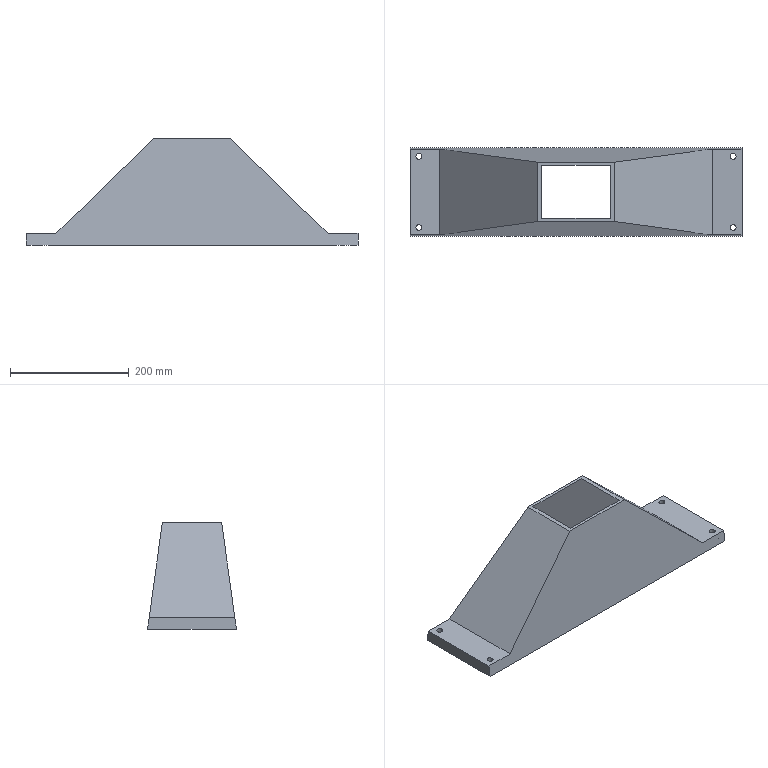Part | SolidWorks | features BaseBody 1 | 1 solid | 34 faces | box 560 x 150 x 180 mm | volume 1083065 mm3 | plane 18 | cylinder 16 | commonest cylinder face diameters 10 x8 25 x8
STEP:
#1=CARTESIAN_POINT('',(260.,-60.,20.));
#2=VERTEX_POINT('',#1);
#3=CARTESIAN_POINT('',(270.,-60.,20.));
#4=VERTEX_POINT('',#3);
#5=CARTESIAN_POINT('',(265.,-60.,20.));
#6=DIRECTION('',(0.,0.,-1.));
#7=DIRECTION('',(1.,0.,0.));
#8=AXIS2_PLACEMENT_3D('',#5,#6,#7);
#9=CIRCLE('',#8,5.);
#10=EDGE_CURVE('',#2,#4,#9,.T.);
#11=ORIENTED_EDGE('',*,*,#10,.F.);
#12=CARTESIAN_POINT('',(260.,-60.,10.));
#13=VERTEX_POINT('',#12);
#14=CARTESIAN_POINT('',(260.,-60.,10.));
#15=DIRECTION('',(0.,0.,-1.));
#16=VECTOR('',#15,1000.);
#17=LINE('',#14,#16);
#18=EDGE_CURVE('',#2,#13,#17,.T.);
#19=ORIENTED_EDGE('',*,*,#18,.T.);
#20=CARTESIAN_POINT('',(270.,-60.,10.));
#21=VERTEX_POINT('',#20);
#22=CARTESIAN_POINT('',(265.,-60.,10.));
#23=DIRECTION('',(0.,0.,1.));
#24=DIRECTION('',(1.,0.,0.));
#25=AXIS2_PLACEMENT_3D('',#22,#23,#24);
#26=CIRCLE('',#25,5.);
#27=EDGE_CURVE('',#21,#13,#26,.T.);
#28=ORIENTED_EDGE('',*,*,#27,.F.);
#29=CARTESIAN_POINT('',(270.,-60.,10.));
#30=DIRECTION('',(0.,0.,-1.));
#31=VECTOR('',#30,1000.);
#32=LINE('',#29,#31);
#33=EDGE_CURVE('',#4,#21,#32,.T.);
#34=ORIENTED_EDGE('',*,*,#33,.F.);
#35=EDGE_LOOP('',(#11,#19,#28,#34));
#36=FACE_OUTER_BOUND('',#35,.T.);
#37=CARTESIAN_POINT('',(265.,-60.,10.));
#38=DIRECTION('',(0.,0.,-1.));
#39=DIRECTION('',(1.,0.,0.));
#40=AXIS2_PLACEMENT_3D('',#37,#38,#39);
#41=CYLINDRICAL_SURFACE('',#40,5.);
#42=ADVANCED_FACE('',(#36),#41,.F.);
#43=CARTESIAN_POINT('',(-270.,60.,20.));
#44=VERTEX_POINT('',#43);
#45=CARTESIAN_POINT('',(-260.,60.,20.));
#46=VERTEX_POINT('',#45);
#47=CARTESIAN_POINT('',(-265.,60.,20.));
#48=DIRECTION('',(0.,0.,-1.));
#49=DIRECTION('',(1.,0.,0.));
#50=AXIS2_PLACEMENT_3D('',#47,#48,#49);
#51=CIRCLE('',#50,5.);
#52=EDGE_CURVE('',#44,#46,#51,.T.);
#53=ORIENTED_EDGE('',*,*,#52,.F.);
#54=CARTESIAN_POINT('',(-270.,60.,10.));
#55=VERTEX_POINT('',#54);
#56=CARTESIAN_POINT('',(-270.,60.,10.));
#57=DIRECTION('',(0.,0.,-1.));
#58=VECTOR('',#57,1000.);
#59=LINE('',#56,#58);
#60=EDGE_CURVE('',#44,#55,#59,.T.);
#61=ORIENTED_EDGE('',*,*,#60,.T.);
#62=CARTESIAN_POINT('',(-260.,60.,10.));
#63=VERTEX_POINT('',#62);
#64=CARTESIAN_POINT('',(-265.,60.,10.));
#65=DIRECTION('',(0.,0.,1.));
#66=DIRECTION('',(1.,0.,0.));
#67=AXIS2_PLACEMENT_3D('',#64,#65,#66);
#68=CIRCLE('',#67,5.);
#69=EDGE_CURVE('',#63,#55,#68,.T.);
#70=ORIENTED_EDGE('',*,*,#69,.F.);
#71=CARTESIAN_POINT('',(-260.,60.,10.));
#72=DIRECTION('',(0.,0.,-1.));
#73=VECTOR('',#72,1000.);
#74=LINE('',#71,#73);
#75=EDGE_CURVE('',#46,#63,#74,.T.);
#76=ORIENTED_EDGE('',*,*,#75,.F.);
#77=EDGE_LOOP('',(#53,#61,#70,#76));
#78=FACE_OUTER_BOUND('',#77,.T.);
#79=CARTESIAN_POINT('',(-265.,60.,10.));
#80=DIRECTION('',(0.,0.,-1.));
#81=DIRECTION('',(1.,0.,0.));
#82=AXIS2_PLACEMENT_3D('',#79,#80,#81);
#83=CYLINDRICAL_SURFACE('',#82,5.);
#84=ADVANCED_FACE('',(#78),#83,.F.);
#85=CARTESIAN_POINT('',(-270.,-60.,20.));
#86=VERTEX_POINT('',#85);
#87=CARTESIAN_POINT('',(-260.,-60.,20.));
#88=VERTEX_POINT('',#87);
#89=CARTESIAN_POINT('',(-265.,-60.,20.));
#90=DIRECTION('',(0.,0.,-1.));
#91=DIRECTION('',(1.,0.,0.));
#92=AXIS2_PLACEMENT_3D('',#89,#90,#91);
#93=CIRCLE('',#92,5.);
#94=EDGE_CURVE('',#86,#88,#93,.T.);
#95=ORIENTED_EDGE('',*,*,#94,.F.);
#96=CARTESIAN_POINT('',(-270.,-60.,10.));
#97=VERTEX_POINT('',#96);
#98=CARTESIAN_POINT('',(-270.,-60.,10.));
#99=DIRECTION('',(0.,0.,-1.));
#100=VECTOR('',#99,1000.);
#101=LINE('',#98,#100);
#102=EDGE_CURVE('',#86,#97,#101,.T.);
#103=ORIENTED_EDGE('',*,*,#102,.T.);
#104=CARTESIAN_POINT('',(-260.,-60.,10.));
#105=VERTEX_POINT('',#104);
#106=CARTESIAN_POINT('',(-265.,-60.,10.));
#107=DIRECTION('',(0.,0.,1.));
#108=DIRECTION('',(1.,0.,0.));
#109=AXIS2_PLACEMENT_3D('',#106,#107,#108);
#110=CIRCLE('',#109,5.);
#111=EDGE_CURVE('',#105,#97,#110,.T.);
#112=ORIENTED_EDGE('',*,*,#111,.F.);
#113=CARTESIAN_POINT('',(-260.,-60.,10.));
#114=DIRECTION('',(0.,0.,-1.));
#115=VECTOR('',#114,1000.);
#116=LINE('',#113,#115);
#117=EDGE_CURVE('',#88,#105,#116,.T.);
#118=ORIENTED_EDGE('',*,*,#117,.F.);
#119=EDGE_LOOP('',(#95,#103,#112,#118));
#120=FACE_OUTER_BOUND('',#119,.T.);
#121=CARTESIAN_POINT('',(-265.,-60.,10.));
#122=DIRECTION('',(0.,0.,-1.));
#123=DIRECTION('',(1.,0.,0.));
#124=AXIS2_PLACEMENT_3D('',#121,#122,#123);
#125=CYLINDRICAL_SURFACE('',#124,5.);
#126=ADVANCED_FACE('',(#120),#125,.F.);
#127=CARTESIAN_POINT('',(260.,60.,20.));
#128=VERTEX_POINT('',#127);
#129=CARTESIAN_POINT('',(270.,60.,20.));
#130=VERTEX_POINT('',#129);
#131=CARTESIAN_POINT('',(265.,60.,20.));
#132=DIRECTION('',(0.,0.,-1.));
#133=DIRECTION('',(1.,0.,0.));
#134=AXIS2_PLACEMENT_3D('',#131,#132,#133);
#135=CIRCLE('',#134,5.);
#136=EDGE_CURVE('',#128,#130,#135,.T.);
#137=ORIENTED_EDGE('',*,*,#136,.F.);
#138=CARTESIAN_POINT('',(260.,60.,10.));
#139=VERTEX_POINT('',#138);
#140=CARTESIAN_POINT('',(260.,60.,10.));
#141=DIRECTION('',(0.,0.,-1.));
#142=VECTOR('',#141,1000.);
#143=LINE('',#140,#142);
#144=EDGE_CURVE('',#128,#139,#143,.T.);
#145=ORIENTED_EDGE('',*,*,#144,.T.);
#146=CARTESIAN_POINT('',(270.,60.,10.));
#147=VERTEX_POINT('',#146);
#148=CARTESIAN_POINT('',(265.,60.,10.));
#149=DIRECTION('',(0.,0.,1.));
#150=DIRECTION('',(1.,0.,0.));
#151=AXIS2_PLACEMENT_3D('',#148,#149,#150);
#152=CIRCLE('',#151,5.);
#153=EDGE_CURVE('',#147,#139,#152,.T.);
#154=ORIENTED_EDGE('',*,*,#153,.F.);
#155=CARTESIAN_POINT('',(270.,60.,10.));
#156=DIRECTION('',(0.,0.,-1.));
#157=VECTOR('',#156,1000.);
#158=LINE('',#155,#157);
#159=EDGE_CURVE('',#130,#147,#158,.T.);
#160=ORIENTED_EDGE('',*,*,#159,.F.);
#161=EDGE_LOOP('',(#137,#145,#154,#160));
#162=FACE_OUTER_BOUND('',#161,.T.);
#163=CARTESIAN_POINT('',(265.,60.,10.));
#164=DIRECTION('',(0.,0.,-1.));
#165=DIRECTION('',(1.,0.,0.));
#166=AXIS2_PLACEMENT_3D('',#163,#164,#165);
#167=CYLINDRICAL_SURFACE('',#166,5.);
#168=ADVANCED_FACE('',(#162),#167,.F.);
#169=CARTESIAN_POINT('',(277.5,60.,10.));
#170=VERTEX_POINT('',#169);
#171=CARTESIAN_POINT('',(252.5,60.,10.));
#172=VERTEX_POINT('',#171);
#173=CARTESIAN_POINT('',(265.,60.,10.));
#174=DIRECTION('',(0.,0.,1.));
#175=DIRECTION('',(1.,0.,0.));
#176=AXIS2_PLACEMENT_3D('',#173,#174,#175);
#177=CIRCLE('',#176,12.5);
#178=EDGE_CURVE('',#170,#172,#177,.T.);
#179=ORIENTED_EDGE('',*,*,#178,.T.);
#180=CARTESIAN_POINT('',(252.5,60.,0.));
#181=VERTEX_POINT('',#180);
#182=CARTESIAN_POINT('',(252.5,60.,0.));
#183=DIRECTION('',(0.,0.,-1.));
#184=VECTOR('',#183,1000.);
#185=LINE('',#182,#184);
#186=EDGE_CURVE('',#172,#181,#185,.T.);
#187=ORIENTED_EDGE('',*,*,#186,.T.);
#188=CARTESIAN_POINT('',(277.5,60.,0.));
#189=VERTEX_POINT('',#188);
#190=CARTESIAN_POINT('',(265.,60.,0.));
#191=DIRECTION('',(0.,0.,1.));
#192=DIRECTION('',(1.,0.,0.));
#193=AXIS2_PLACEMENT_3D('',#190,#191,#192);
#194=CIRCLE('',#193,12.5);
#195=EDGE_CURVE('',#189,#181,#194,.T.);
#196=ORIENTED_EDGE('',*,*,#195,.F.);
#197=CARTESIAN_POINT('',(277.5,60.,0.));
#198=DIRECTION('',(0.,0.,-1.));
#199=VECTOR('',#198,1000.);
#200=LINE('',#197,#199);
#201=EDGE_CURVE('',#170,#189,#200,.T.);
#202=ORIENTED_EDGE('',*,*,#201,.F.);
#203=EDGE_LOOP('',(#179,#187,#196,#202));
#204=FACE_OUTER_BOUND('',#203,.T.);
#205=CARTESIAN_POINT('',(265.,60.,0.));
#206=DIRECTION('',(0.,0.,-1.));
#207=DIRECTION('',(1.,0.,0.));
#208=AXIS2_PLACEMENT_3D('',#205,#206,#207);
#209=CYLINDRICAL_SURFACE('',#208,12.5);
#210=ADVANCED_FACE('',(#204),#209,.F.);
#211=CARTESIAN_POINT('',(-252.5,60.,10.));
#212=VERTEX_POINT('',#211);
#213=CARTESIAN_POINT('',(-277.5,60.,10.));
#214=VERTEX_POINT('',#213);
#215=CARTESIAN_POINT('',(-265.,60.,10.));
#216=DIRECTION('',(0.,0.,1.));
#217=DIRECTION('',(1.,0.,0.));
#218=AXIS2_PLACEMENT_3D('',#215,#216,#217);
#219=CIRCLE('',#218,12.5);
#220=EDGE_CURVE('',#212,#214,#219,.T.);
#221=ORIENTED_EDGE('',*,*,#220,.T.);
#222=CARTESIAN_POINT('',(-277.5,60.,0.));
#223=VERTEX_POINT('',#222);
#224=CARTESIAN_POINT('',(-277.5,60.,0.));
#225=DIRECTION('',(0.,0.,-1.));
#226=VECTOR('',#225,1000.);
#227=LINE('',#224,#226);
#228=EDGE_CURVE('',#214,#223,#227,.T.);
#229=ORIENTED_EDGE('',*,*,#228,.T.);
#230=CARTESIAN_POINT('',(-252.5,60.,0.));
#231=VERTEX_POINT('',#230);
#232=CARTESIAN_POINT('',(-265.,60.,0.));
#233=DIRECTION('',(0.,0.,1.));
#234=DIRECTION('',(1.,0.,0.));
#235=AXIS2_PLACEMENT_3D('',#232,#233,#234);
#236=CIRCLE('',#235,12.5);
#237=EDGE_CURVE('',#231,#223,#236,.T.);
#238=ORIENTED_EDGE('',*,*,#237,.F.);
#239=CARTESIAN_POINT('',(-252.5,60.,0.));
#240=DIRECTION('',(0.,0.,-1.));
#241=VECTOR('',#240,1000.);
#242=LINE('',#239,#241);
#243=EDGE_CURVE('',#212,#231,#242,.T.);
#244=ORIENTED_EDGE('',*,*,#243,.F.);
#245=EDGE_LOOP('',(#221,#229,#238,#244));
#246=FACE_OUTER_BOUND('',#245,.T.);
#247=CARTESIAN_POINT('',(-265.,60.,0.));
#248=DIRECTION('',(0.,0.,-1.));
#249=DIRECTION('',(1.,0.,0.));
#250=AXIS2_PLACEMENT_3D('',#247,#248,#249);
#251=CYLINDRICAL_SURFACE('',#250,12.5);
#252=ADVANCED_FACE('',(#246),#251,.F.);
#253=CARTESIAN_POINT('',(-252.5,-60.,10.));
#254=VERTEX_POINT('',#253);
#255=CARTESIAN_POINT('',(-277.5,-60.,10.));
#256=VERTEX_POINT('',#255);
#257=CARTESIAN_POINT('',(-265.,-60.,10.));
#258=DIRECTION('',(0.,0.,1.));
#259=DIRECTION('',(1.,0.,0.));
#260=AXIS2_PLACEMENT_3D('',#257,#258,#259);
#261=CIRCLE('',#260,12.5);
#262=EDGE_CURVE('',#254,#256,#261,.T.);
#263=ORIENTED_EDGE('',*,*,#262,.T.);
#264=CARTESIAN_POINT('',(-277.5,-60.,0.));
#265=VERTEX_POINT('',#264);
#266=CARTESIAN_POINT('',(-277.5,-60.,0.));
#267=DIRECTION('',(0.,0.,-1.));
#268=VECTOR('',#267,1000.);
#269=LINE('',#266,#268);
#270=EDGE_CURVE('',#256,#265,#269,.T.);
#271=ORIENTED_EDGE('',*,*,#270,.T.);
#272=CARTESIAN_POINT('',(-252.5,-60.,0.));
#273=VERTEX_POINT('',#272);
#274=CARTESIAN_POINT('',(-265.,-60.,0.));
#275=DIRECTION('',(0.,0.,1.));
#276=DIRECTION('',(1.,0.,0.));
#277=AXIS2_PLACEMENT_3D('',#274,#275,#276);
#278=CIRCLE('',#277,12.5);
#279=EDGE_CURVE('',#273,#265,#278,.T.);
#280=ORIENTED_EDGE('',*,*,#279,.F.);
#281=CARTESIAN_POINT('',(-252.5,-60.,0.));
#282=DIRECTION('',(0.,0.,-1.));
#283=VECTOR('',#282,1000.);
#284=LINE('',#281,#283);
#285=EDGE_CURVE('',#254,#273,#284,.T.);
#286=ORIENTED_EDGE('',*,*,#285,.F.);
#287=EDGE_LOOP('',(#263,#271,#280,#286));
#288=FACE_OUTER_BOUND('',#287,.T.);
#289=CARTESIAN_POINT('',(-265.,-60.,0.));
#290=DIRECTION('',(0.,0.,-1.));
#291=DIRECTION('',(1.,0.,0.));
#292=AXIS2_PLACEMENT_3D('',#289,#290,#291);
#293=CYLINDRICAL_SURFACE('',#292,12.5);
#294=ADVANCED_FACE('',(#288),#293,.F.);
#295=CARTESIAN_POINT('',(277.5,-60.,10.));
#296=VERTEX_POINT('',#295);
#297=CARTESIAN_POINT('',(252.5,-60.,10.));
#298=VERTEX_POINT('',#297);
#299=CARTESIAN_POINT('',(265.,-60.,10.));
#300=DIRECTION('',(0.,0.,1.));
#301=DIRECTION('',(1.,0.,0.));
#302=AXIS2_PLACEMENT_3D('',#299,#300,#301);
#303=CIRCLE('',#302,12.5);
#304=EDGE_CURVE('',#296,#298,#303,.T.);
#305=ORIENTED_EDGE('',*,*,#304,.T.);
#306=CARTESIAN_POINT('',(252.5,-60.,0.));
#307=VERTEX_POINT('',#306);
#308=CARTESIAN_POINT('',(252.5,-60.,0.));
#309=DIRECTION('',(0.,0.,-1.));
#310=VECTOR('',#309,1000.);
#311=LINE('',#308,#310);
#312=EDGE_CURVE('',#298,#307,#311,.T.);
#313=ORIENTED_EDGE('',*,*,#312,.T.);
#314=CARTESIAN_POINT('',(277.5,-60.,0.));
#315=VERTEX_POINT('',#314);
#316=CARTESIAN_POINT('',(265.,-60.,0.));
#317=DIRECTION('',(0.,0.,1.));
#318=DIRECTION('',(1.,0.,0.));
#319=AXIS2_PLACEMENT_3D('',#316,#317,#318);
#320=CIRCLE('',#319,12.5);
#321=EDGE_CURVE('',#315,#307,#320,.T.);
#322=ORIENTED_EDGE('',*,*,#321,.F.);
#323=CARTESIAN_POINT('',(277.5,-60.,0.));
#324=DIRECTION('',(0.,0.,-1.));
#325=VECTOR('',#324,1000.);
#326=LINE('',#323,#325);
#327=EDGE_CURVE('',#296,#315,#326,.T.);
#328=ORIENTED_EDGE('',*,*,#327,.F.);
#329=EDGE_LOOP('',(#305,#313,#322,#328));
#330=FACE_OUTER_BOUND('',#329,.T.);
#331=CARTESIAN_POINT('',(265.,-60.,0.));
#332=DIRECTION('',(0.,0.,-1.));
#333=DIRECTION('',(1.,0.,0.));
#334=AXIS2_PLACEMENT_3D('',#331,#332,#333);
#335=CYLINDRICAL_SURFACE('',#334,12.5);
#336=ADVANCED_FACE('',(#330),#335,.F.);
#337=ORIENTED_EDGE('',*,*,#153,.T.);
#338=CARTESIAN_POINT('',(265.,60.,10.));
#339=DIRECTION('',(0.,0.,1.));
#340=DIRECTION('',(1.,0.,0.));
#341=AXIS2_PLACEMENT_3D('',#338,#339,#340);
#342=CIRCLE('',#341,5.);
#343=EDGE_CURVE('',#139,#147,#342,.T.);
#344=ORIENTED_EDGE('',*,*,#343,.T.);
#345=EDGE_LOOP('',(#337,#344));
#346=FACE_BOUND('',#345,.T.);
#347=ORIENTED_EDGE('',*,*,#178,.F.);
#348=CARTESIAN_POINT('',(265.,60.,10.));
#349=DIRECTION('',(0.,0.,1.));
#350=DIRECTION('',(1.,0.,0.));
#351=AXIS2_PLACEMENT_3D('',#348,#349,#350);
#352=CIRCLE('',#351,12.5);
#353=EDGE_CURVE('',#172,#170,#352,.T.);
#354=ORIENTED_EDGE('',*,*,#353,.F.);
#355=EDGE_LOOP('',(#347,#354));
#356=FACE_OUTER_BOUND('',#355,.T.);
#357=CARTESIAN_POINT('',(265.,60.,10.));
#358=DIRECTION('',(0.,0.,1.));
#359=DIRECTION('',(1.,0.,0.));
#360=AXIS2_PLACEMENT_3D('',#357,#358,#359);
#361=PLANE('',#360);
#362=ADVANCED_FACE('',(#346,#356),#361,.F.);
#363=ORIENTED_EDGE('',*,*,#69,.T.);
#364=CARTESIAN_POINT('',(-265.,60.,10.));
#365=DIRECTION('',(0.,0.,1.));
#366=DIRECTION('',(1.,0.,0.));
#367=AXIS2_PLACEMENT_3D('',#364,#365,#366);
#368=CIRCLE('',#367,5.);
#369=EDGE_CURVE('',#55,#63,#368,.T.);
#370=ORIENTED_EDGE('',*,*,#369,.T.);
#371=EDGE_LOOP('',(#363,#370));
#372=FACE_BOUND('',#371,.T.);
#373=ORIENTED_EDGE('',*,*,#220,.F.);
#374=CARTESIAN_POINT('',(-265.,60.,10.));
#375=DIRECTION('',(0.,0.,1.));
#376=DIRECTION('',(1.,0.,0.));
#377=AXIS2_PLACEMENT_3D('',#374,#375,#376);
#378=CIRCLE('',#377,12.5);
#379=EDGE_CURVE('',#214,#212,#378,.T.);
#380=ORIENTED_EDGE('',*,*,#379,.F.);
#381=EDGE_LOOP('',(#373,#380));
#382=FACE_OUTER_BOUND('',#381,.T.);
#383=CARTESIAN_POINT('',(-265.,60.,10.));
#384=DIRECTION('',(0.,0.,1.));
#385=DIRECTION('',(1.,0.,0.));
#386=AXIS2_PLACEMENT_3D('',#383,#384,#385);
#387=PLANE('',#386);
#388=ADVANCED_FACE('',(#372,#382),#387,.F.);
#389=ORIENTED_EDGE('',*,*,#111,.T.);
#390=CARTESIAN_POINT('',(-265.,-60.,10.));
#391=DIRECTION('',(0.,0.,1.));
#392=DIRECTION('',(1.,0.,0.));
#393=AXIS2_PLACEMENT_3D('',#390,#391,#392);
#394=CIRCLE('',#393,5.);
#395=EDGE_CURVE('',#97,#105,#394,.T.);
#396=ORIENTED_EDGE('',*,*,#395,.T.);
#397=EDGE_LOOP('',(#389,#396));
#398=FACE_BOUND('',#397,.T.);
#399=ORIENTED_EDGE('',*,*,#262,.F.);
#400=CARTESIAN_POINT('',(-265.,-60.,10.));
#401=DIRECTION('',(0.,0.,1.));
#402=DIRECTION('',(1.,0.,0.));
#403=AXIS2_PLACEMENT_3D('',#400,#401,#402);
#404=CIRCLE('',#403,12.5);
#405=EDGE_CURVE('',#256,#254,#404,.T.);
#406=ORIENTED_EDGE('',*,*,#405,.F.);
#407=EDGE_LOOP('',(#399,#406));
#408=FACE_OUTER_BOUND('',#407,.T.);
#409=CARTESIAN_POINT('',(-265.,-60.,10.));
#410=DIRECTION('',(0.,0.,1.));
#411=DIRECTION('',(1.,0.,0.));
#412=AXIS2_PLACEMENT_3D('',#409,#410,#411);
#413=PLANE('',#412);
#414=ADVANCED_FACE('',(#398,#408),#413,.F.);
#415=ORIENTED_EDGE('',*,*,#27,.T.);
#416=CARTESIAN_POINT('',(265.,-60.,10.));
#417=DIRECTION('',(0.,0.,1.));
#418=DIRECTION('',(1.,0.,0.));
#419=AXIS2_PLACEMENT_3D('',#416,#417,#418);
#420=CIRCLE('',#419,5.);
#421=EDGE_CURVE('',#13,#21,#420,.T.);
#422=ORIENTED_EDGE('',*,*,#421,.T.);
#423=EDGE_LOOP('',(#415,#422));
#424=FACE_BOUND('',#423,.T.);
#425=ORIENTED_EDGE('',*,*,#304,.F.);
#426=CARTESIAN_POINT('',(265.,-60.,10.));
#427=DIRECTION('',(0.,0.,1.));
#428=DIRECTION('',(1.,0.,0.));
#429=AXIS2_PLACEMENT_3D('',#426,#427,#428);
#430=CIRCLE('',#429,12.5);
#431=EDGE_CURVE('',#298,#296,#430,.T.);
#432=ORIENTED_EDGE('',*,*,#431,.F.);
#433=EDGE_LOOP('',(#425,#432));
#434=FACE_OUTER_BOUND('',#433,.T.);
#435=CARTESIAN_POINT('',(265.,-60.,10.));
#436=DIRECTION('',(0.,0.,1.));
#437=DIRECTION('',(1.,0.,0.));
#438=AXIS2_PLACEMENT_3D('',#435,#436,#437);
#439=PLANE('',#438);
#440=ADVANCED_FACE('',(#424,#434),#439,.F.);
#441=CARTESIAN_POINT('',(280.,-72.222,20.));
#442=VERTEX_POINT('',#441);
#443=CARTESIAN_POINT('',(280.,-75.,0.));
#444=VERTEX_POINT('',#443);
#445=CARTESIAN_POINT('',(280.,-73.611,10.));
#446=DIRECTION('',(0.,-0.1376,-0.9905));
#447=VECTOR('',#446,1000.);
#448=LINE('',#445,#447);
#449=EDGE_CURVE('',#442,#444,#448,.T.);
#450=ORIENTED_EDGE('',*,*,#449,.T.);
#451=CARTESIAN_POINT('',(280.,75.,0.));
#452=VERTEX_POINT('',#451);
#453=CARTESIAN_POINT('',(280.,75.,0.));
#454=DIRECTION('',(0.,-1.,0.));
#455=VECTOR('',#454,1000.);
#456=LINE('',#453,#455);
#457=EDGE_CURVE('',#452,#444,#456,.T.);
#458=ORIENTED_EDGE('',*,*,#457,.F.);
#459=CARTESIAN_POINT('',(280.,72.222,20.));
#460=VERTEX_POINT('',#459);
#461=CARTESIAN_POINT('',(280.,73.581,10.22));
#462=DIRECTION('',(0.,-0.1376,0.9905));
#463=VECTOR('',#462,1000.);
#464=LINE('',#461,#463);
#465=EDGE_CURVE('',#452,#460,#464,.T.);
#466=ORIENTED_EDGE('',*,*,#465,.T.);
#467=CARTESIAN_POINT('',(280.,75.,20.));
#468=DIRECTION('',(0.,1.,0.));
#469=VECTOR('',#468,1000.);
#470=LINE('',#467,#469);
#471=EDGE_CURVE('',#442,#460,#470,.T.);
#472=ORIENTED_EDGE('',*,*,#471,.F.);
#473=EDGE_LOOP('',(#450,#458,#466,#472));
#474=FACE_OUTER_BOUND('',#473,.T.);
#475=CARTESIAN_POINT('',(280.,-75.,0.));
#476=DIRECTION('',(1.,0.,0.));
#477=DIRECTION('',(0.,-1.,0.));
#478=AXIS2_PLACEMENT_3D('',#475,#476,#477);
#479=PLANE('',#478);
#480=ADVANCED_FACE('',(#474),#479,.T.);
#481=CARTESIAN_POINT('',(-229.444,72.222,20.));
#482=VERTEX_POINT('',#481);
#483=CARTESIAN_POINT('',(-65.,50.,180.));
#484=VERTEX_POINT('',#483);
#485=CARTESIAN_POINT('',(-250.,75.,0.));
#486=DIRECTION('',(0.7134,-0.0964,0.6941));
#487=VECTOR('',#486,1000.);
#488=LINE('',#485,#487);
#489=EDGE_CURVE('',#482,#484,#488,.T.);
#490=ORIENTED_EDGE('',*,*,#489,.T.);
#491=CARTESIAN_POINT('',(65.,50.,180.));
#492=VERTEX_POINT('',#491);
#493=CARTESIAN_POINT('',(-65.,50.,180.));
#494=DIRECTION('',(1.,0.,0.));
#495=VECTOR('',#494,1000.);
#496=LINE('',#493,#495);
#497=EDGE_CURVE('',#484,#492,#496,.T.);
#498=ORIENTED_EDGE('',*,*,#497,.T.);
#499=CARTESIAN_POINT('',(229.444,72.222,20.));
#500=VERTEX_POINT('',#499);
#501=CARTESIAN_POINT('',(250.,75.,0.));
#502=DIRECTION('',(-0.7134,-0.0964,0.6941));
#503=VECTOR('',#502,1000.);
#504=LINE('',#501,#503);
#505=EDGE_CURVE('',#500,#492,#504,.T.);
#506=ORIENTED_EDGE('',*,*,#505,.F.);
#507=CARTESIAN_POINT('',(140.,72.222,20.));
#508=DIRECTION('',(-1.,0.,0.));
#509=VECTOR('',#508,1000.);
#510=LINE('',#507,#509);
#511=EDGE_CURVE('',#460,#500,#510,.T.);
#512=ORIENTED_EDGE('',*,*,#511,.F.);
#513=ORIENTED_EDGE('',*,*,#465,.F.);
#514=CARTESIAN_POINT('',(-280.,75.,0.));
#515=VERTEX_POINT('',#514);
#516=CARTESIAN_POINT('',(-280.,75.,0.));
#517=DIRECTION('',(1.,0.,0.));
#518=VECTOR('',#517,1000.);
#519=LINE('',#516,#518);
#520=EDGE_CURVE('',#515,#452,#519,.T.);
#521=ORIENTED_EDGE('',*,*,#520,.F.);
#522=CARTESIAN_POINT('',(-280.,72.222,20.));
#523=VERTEX_POINT('',#522);
#524=CARTESIAN_POINT('',(-280.,75.,0.));
#525=DIRECTION('',(0.,0.1376,-0.9905));
#526=VECTOR('',#525,1000.);
#527=LINE('',#524,#526);
#528=EDGE_CURVE('',#523,#515,#527,.T.);
#529=ORIENTED_EDGE('',*,*,#528,.F.);
#530=CARTESIAN_POINT('',(140.,72.222,20.));
#531=DIRECTION('',(-1.,0.,0.));
#532=VECTOR('',#531,1000.);
#533=LINE('',#530,#532);
#534=EDGE_CURVE('',#482,#523,#533,.T.);
#535=ORIENTED_EDGE('',*,*,#534,.F.);
#536=EDGE_LOOP('',(#490,#498,#506,#512,#513,#521,#529,#535));
#537=FACE_OUTER_BOUND('',#536,.T.);
#538=CARTESIAN_POINT('',(-250.,75.,0.));
#539=DIRECTION('',(0.,-0.9905,-0.1376));
#540=DIRECTION('',(0.,0.1376,-0.9905));
#541=AXIS2_PLACEMENT_3D('',#538,#539,#540);
#542=PLANE('',#541);
#543=ADVANCED_FACE('',(#537),#542,.F.);
#544=CARTESIAN_POINT('',(-265.,60.,20.));
#545=DIRECTION('',(0.,0.,-1.));
#546=DIRECTION('',(1.,0.,0.));
#547=AXIS2_PLACEMENT_3D('',#544,#545,#546);
#548=CIRCLE('',#547,5.);
#549=EDGE_CURVE('',#46,#44,#548,.T.);
#550=ORIENTED_EDGE('',*,*,#549,.T.);
#551=ORIENTED_EDGE('',*,*,#52,.T.);
#552=EDGE_LOOP('',(#550,#551));
#553=FACE_BOUND('',#552,.T.);
#554=CARTESIAN_POINT('',(-265.,-60.,20.));
#555=DIRECTION('',(0.,0.,-1.));
#556=DIRECTION('',(1.,0.,0.));
#557=AXIS2_PLACEMENT_3D('',#554,#555,#556);
#558=CIRCLE('',#557,5.);
#559=EDGE_CURVE('',#88,#86,#558,.T.);
#560=ORIENTED_EDGE('',*,*,#559,.T.);
#561=ORIENTED_EDGE('',*,*,#94,.T.);
#562=EDGE_LOOP('',(#560,#561));
#563=FACE_BOUND('',#562,.T.);
#564=CARTESIAN_POINT('',(-280.,-72.222,20.));
#565=VERTEX_POINT('',#564);
#566=CARTESIAN_POINT('',(-229.444,-72.222,20.));
#567=VERTEX_POINT('',#566);
#568=CARTESIAN_POINT('',(140.,-72.222,20.));
#569=DIRECTION('',(1.,0.,0.));
#570=VECTOR('',#569,1000.);
#571=LINE('',#568,#570);
#572=EDGE_CURVE('',#565,#567,#571,.T.);
#573=ORIENTED_EDGE('',*,*,#572,.T.);
#574=CARTESIAN_POINT('',(-229.444,0.,20.));
#575=DIRECTION('',(0.,-1.,0.));
#576=VECTOR('',#575,1000.);
#577=LINE('',#574,#576);
#578=EDGE_CURVE('',#482,#567,#577,.T.);
#579=ORIENTED_EDGE('',*,*,#578,.F.);
#580=ORIENTED_EDGE('',*,*,#534,.T.);
#581=CARTESIAN_POINT('',(-280.,-75.,20.));
#582=DIRECTION('',(0.,-1.,0.));
#583=VECTOR('',#582,1000.);
#584=LINE('',#581,#583);
#585=EDGE_CURVE('',#523,#565,#584,.T.);
#586=ORIENTED_EDGE('',*,*,#585,.T.);
#587=EDGE_LOOP('',(#573,#579,#580,#586));
#588=FACE_OUTER_BOUND('',#587,.T.);
#589=CARTESIAN_POINT('',(0.,0.,20.));
#590=DIRECTION('',(0.,0.,1.));
#591=DIRECTION('',(1.,0.,0.));
#592=AXIS2_PLACEMENT_3D('',#589,#590,#591);
#593=PLANE('',#592);
#594=ADVANCED_FACE('',(#553,#563,#588),#593,.T.);
#595=CARTESIAN_POINT('',(-280.,-75.,0.));
#596=VERTEX_POINT('',#595);
#597=CARTESIAN_POINT('',(-280.,-72.192,20.22));
#598=DIRECTION('',(0.,0.1376,0.9905));
#599=VECTOR('',#598,1000.);
#600=LINE('',#597,#599);
#601=EDGE_CURVE('',#596,#565,#600,.T.);
#602=ORIENTED_EDGE('',*,*,#601,.T.);
#603=ORIENTED_EDGE('',*,*,#585,.F.);
#604=ORIENTED_EDGE('',*,*,#528,.T.);
#605=CARTESIAN_POINT('',(-280.,-75.,0.));
#606=DIRECTION('',(0.,1.,0.));
#607=VECTOR('',#606,1000.);
#608=LINE('',#605,#607);
#609=EDGE_CURVE('',#596,#515,#608,.T.);
#610=ORIENTED_EDGE('',*,*,#609,.F.);
#611=EDGE_LOOP('',(#602,#603,#604,#610));
#612=FACE_OUTER_BOUND('',#611,.T.);
#613=CARTESIAN_POINT('',(-280.,75.,0.));
#614=DIRECTION('',(-1.,0.,0.));
#615=DIRECTION('',(0.,0.,1.));
#616=AXIS2_PLACEMENT_3D('',#613,#614,#615);
#617=PLANE('',#616);
#618=ADVANCED_FACE('',(#612),#617,.T.);
#619=CARTESIAN_POINT('',(229.444,-72.222,20.));
#620=VERTEX_POINT('',#619);
#621=CARTESIAN_POINT('',(229.444,75.,20.));
#622=DIRECTION('',(0.,1.,0.));
#623=VECTOR('',#622,1000.);
#624=LINE('',#621,#623);
#625=EDGE_CURVE('',#620,#500,#624,.T.);
#626=ORIENTED_EDGE('',*,*,#625,.T.);
#627=ORIENTED_EDGE('',*,*,#505,.T.);
#628=CARTESIAN_POINT('',(65.,-50.,180.));
#629=VERTEX_POINT('',#628);
#630=CARTESIAN_POINT('',(65.,50.,180.));
#631=DIRECTION('',(0.,-1.,0.));
#632=VECTOR('',#631,1000.);
#633=LINE('',#630,#632);
#634=EDGE_CURVE('',#492,#629,#633,.T.);
#635=ORIENTED_EDGE('',*,*,#634,.T.);
#636=CARTESIAN_POINT('',(250.,-75.,0.));
#637=DIRECTION('',(-0.7134,0.0964,0.6941));
#638=VECTOR('',#637,1000.);
#639=LINE('',#636,#638);
#640=EDGE_CURVE('',#620,#629,#639,.T.);
#641=ORIENTED_EDGE('',*,*,#640,.F.);
#642=EDGE_LOOP('',(#626,#627,#635,#641));
#643=FACE_OUTER_BOUND('',#642,.T.);
#644=CARTESIAN_POINT('',(250.,75.,0.));
#645=DIRECTION('',(-0.6974,0.,-0.7167));
#646=DIRECTION('',(-0.7167,0.,0.6974));
#647=AXIS2_PLACEMENT_3D('',#644,#645,#646);
#648=PLANE('',#647);
#649=ADVANCED_FACE('',(#643),#648,.F.);
#650=CARTESIAN_POINT('',(265.,-60.,20.));
#651=DIRECTION('',(0.,0.,-1.));
#652=DIRECTION('',(1.,0.,0.));
#653=AXIS2_PLACEMENT_3D('',#650,#651,#652);
#654=CIRCLE('',#653,5.);
#655=EDGE_CURVE('',#4,#2,#654,.T.);
#656=ORIENTED_EDGE('',*,*,#655,.T.);
#657=ORIENTED_EDGE('',*,*,#10,.T.);
#658=EDGE_LOOP('',(#656,#657));
#659=FACE_BOUND('',#658,.T.);
#660=CARTESIAN_POINT('',(265.,60.,20.));
#661=DIRECTION('',(0.,0.,-1.));
#662=DIRECTION('',(1.,0.,0.));
#663=AXIS2_PLACEMENT_3D('',#660,#661,#662);
#664=CIRCLE('',#663,5.);
#665=EDGE_CURVE('',#130,#128,#664,.T.);
#666=ORIENTED_EDGE('',*,*,#665,.T.);
#667=ORIENTED_EDGE('',*,*,#136,.T.);
#668=EDGE_LOOP('',(#666,#667));
#669=FACE_BOUND('',#668,.T.);
#670=CARTESIAN_POINT('',(140.,-72.222,20.));
#671=DIRECTION('',(1.,0.,0.));
#672=VECTOR('',#671,1000.);
#673=LINE('',#670,#672);
#674=EDGE_CURVE('',#620,#442,#673,.T.);
#675=ORIENTED_EDGE('',*,*,#674,.T.);
#676=ORIENTED_EDGE('',*,*,#471,.T.);
#677=ORIENTED_EDGE('',*,*,#511,.T.);
#678=ORIENTED_EDGE('',*,*,#625,.F.);
#679=EDGE_LOOP('',(#675,#676,#677,#678));
#680=FACE_OUTER_BOUND('',#679,.T.);
#681=CARTESIAN_POINT('',(0.,0.,20.));
#682=DIRECTION('',(0.,0.,1.));
#683=DIRECTION('',(1.,0.,0.));
#684=AXIS2_PLACEMENT_3D('',#681,#682,#683);
#685=PLANE('',#684);
#686=ADVANCED_FACE('',(#659,#669,#680),#685,.T.);
#687=ORIENTED_EDGE('',*,*,#578,.T.);
#688=CARTESIAN_POINT('',(-65.,-50.,180.));
#689=VERTEX_POINT('',#688);
#690=CARTESIAN_POINT('',(-250.,-75.,0.));
#691=DIRECTION('',(0.7134,0.0964,0.6941));
#692=VECTOR('',#691,1000.);
#693=LINE('',#690,#692);
#694=EDGE_CURVE('',#567,#689,#693,.T.);
#695=ORIENTED_EDGE('',*,*,#694,.T.);
#696=CARTESIAN_POINT('',(-65.,-50.,180.));
#697=DIRECTION('',(0.,1.,0.));
#698=VECTOR('',#697,1000.);
#699=LINE('',#696,#698);
#700=EDGE_CURVE('',#689,#484,#699,.T.);
#701=ORIENTED_EDGE('',*,*,#700,.T.);
#702=ORIENTED_EDGE('',*,*,#489,.F.);
#703=EDGE_LOOP('',(#687,#695,#701,#702));
#704=FACE_OUTER_BOUND('',#703,.T.);
#705=CARTESIAN_POINT('',(-250.,-75.,0.));
#706=DIRECTION('',(0.6974,0.,-0.7167));
#707=DIRECTION('',(0.,-1.,0.));
#708=AXIS2_PLACEMENT_3D('',#705,#706,#707);
#709=PLANE('',#708);
#710=ADVANCED_FACE('',(#704),#709,.F.);
#711=ORIENTED_EDGE('',*,*,#195,.T.);
#712=CARTESIAN_POINT('',(265.,60.,0.));
#713=DIRECTION('',(0.,0.,1.));
#714=DIRECTION('',(1.,0.,0.));
#715=AXIS2_PLACEMENT_3D('',#712,#713,#714);
#716=CIRCLE('',#715,12.5);
#717=EDGE_CURVE('',#181,#189,#716,.T.);
#718=ORIENTED_EDGE('',*,*,#717,.T.);
#719=EDGE_LOOP('',(#711,#718));
#720=FACE_BOUND('',#719,.T.);
#721=ORIENTED_EDGE('',*,*,#237,.T.);
#722=CARTESIAN_POINT('',(-265.,60.,0.));
#723=DIRECTION('',(0.,0.,1.));
#724=DIRECTION('',(1.,0.,0.));
#725=AXIS2_PLACEMENT_3D('',#722,#723,#724);
#726=CIRCLE('',#725,12.5);
#727=EDGE_CURVE('',#223,#231,#726,.T.);
#728=ORIENTED_EDGE('',*,*,#727,.T.);
#729=EDGE_LOOP('',(#721,#728));
#730=FACE_BOUND('',#729,.T.);
#731=ORIENTED_EDGE('',*,*,#279,.T.);
#732=CARTESIAN_POINT('',(-265.,-60.,0.));
#733=DIRECTION('',(0.,0.,1.));
#734=DIRECTION('',(1.,0.,0.));
#735=AXIS2_PLACEMENT_3D('',#732,#733,#734);
#736=CIRCLE('',#735,12.5);
#737=EDGE_CURVE('',#265,#273,#736,.T.);
#738=ORIENTED_EDGE('',*,*,#737,.T.);
#739=EDGE_LOOP('',(#731,#738));
#740=FACE_BOUND('',#739,.T.);
#741=ORIENTED_EDGE('',*,*,#321,.T.);
#742=CARTESIAN_POINT('',(265.,-60.,0.));
#743=DIRECTION('',(0.,0.,1.));
#744=DIRECTION('',(1.,0.,0.));
#745=AXIS2_PLACEMENT_3D('',#742,#743,#744);
#746=CIRCLE('',#745,12.5);
#747=EDGE_CURVE('',#307,#315,#746,.T.);
#748=ORIENTED_EDGE('',*,*,#747,.T.);
#749=EDGE_LOOP('',(#741,#748));
#750=FACE_BOUND('',#749,.T.);
#751=CARTESIAN_POINT('',(242.83,69.952,0.));
#752=VERTEX_POINT('',#751);
#753=CARTESIAN_POINT('',(-242.83,69.952,0.));
#754=VERTEX_POINT('',#753);
#755=CARTESIAN_POINT('',(-125.,69.952,0.));
#756=DIRECTION('',(-1.,0.,0.));
#757=VECTOR('',#756,1000.);
#758=LINE('',#755,#757);
#759=EDGE_CURVE('',#752,#754,#758,.T.);
#760=ORIENTED_EDGE('',*,*,#759,.T.);
#761=CARTESIAN_POINT('',(-242.83,-69.952,0.));
#762=VERTEX_POINT('',#761);
#763=CARTESIAN_POINT('',(-242.83,-37.5,0.));
#764=DIRECTION('',(0.,-1.,0.));
#765=VECTOR('',#764,1000.);
#766=LINE('',#763,#765);
#767=EDGE_CURVE('',#754,#762,#766,.T.);
#768=ORIENTED_EDGE('',*,*,#767,.T.);
#769=CARTESIAN_POINT('',(242.83,-69.952,0.));
#770=VERTEX_POINT('',#769);
#771=CARTESIAN_POINT('',(125.,-69.952,0.));
#772=DIRECTION('',(1.,0.,0.));
#773=VECTOR('',#772,1000.);
#774=LINE('',#771,#773);
#775=EDGE_CURVE('',#762,#770,#774,.T.);
#776=ORIENTED_EDGE('',*,*,#775,.T.);
#777=CARTESIAN_POINT('',(242.83,37.5,0.));
#778=DIRECTION('',(0.,1.,0.));
#779=VECTOR('',#778,1000.);
#780=LINE('',#777,#779);
#781=EDGE_CURVE('',#770,#752,#780,.T.);
#782=ORIENTED_EDGE('',*,*,#781,.T.);
#783=EDGE_LOOP('',(#760,#768,#776,#782));
#784=FACE_BOUND('',#783,.T.);
#785=ORIENTED_EDGE('',*,*,#520,.T.);
#786=ORIENTED_EDGE('',*,*,#457,.T.);
#787=CARTESIAN_POINT('',(280.,-75.,0.));
#788=DIRECTION('',(-1.,0.,0.));
#789=VECTOR('',#788,1000.);
#790=LINE('',#787,#789);
#791=EDGE_CURVE('',#444,#596,#790,.T.);
#792=ORIENTED_EDGE('',*,*,#791,.T.);
#793=ORIENTED_EDGE('',*,*,#609,.T.);
#794=EDGE_LOOP('',(#785,#786,#792,#793));
#795=FACE_OUTER_BOUND('',#794,.T.);
#796=CARTESIAN_POINT('',(0.,0.,0.));
#797=DIRECTION('',(0.,0.,1.));
#798=DIRECTION('',(1.,0.,0.));
#799=AXIS2_PLACEMENT_3D('',#796,#797,#798);
#800=PLANE('',#799);
#801=ADVANCED_FACE('',(#720,#730,#740,#750,#784,#795),#800,.F.);
#802=ORIENTED_EDGE('',*,*,#759,.F.);
#803=CARTESIAN_POINT('',(57.83,44.952,180.));
#804=VERTEX_POINT('',#803);
#805=CARTESIAN_POINT('',(119.596,53.299,119.904));
#806=DIRECTION('',(-0.7134,-0.0964,0.6941));
#807=VECTOR('',#806,1000.);
#808=LINE('',#805,#807);
#809=EDGE_CURVE('',#752,#804,#808,.T.);
#810=ORIENTED_EDGE('',*,*,#809,.T.);
#811=CARTESIAN_POINT('',(-57.83,44.952,180.));
#812=VERTEX_POINT('',#811);
#813=CARTESIAN_POINT('',(-125.,44.952,180.));
#814=DIRECTION('',(1.,0.,0.));
#815=VECTOR('',#814,1000.);
#816=LINE('',#813,#815);
#817=EDGE_CURVE('',#812,#804,#816,.T.);
#818=ORIENTED_EDGE('',*,*,#817,.F.);
#819=CARTESIAN_POINT('',(-241.668,69.795,1.13));
#820=DIRECTION('',(0.7134,-0.0964,0.6941));
#821=VECTOR('',#820,1000.);
#822=LINE('',#819,#821);
#823=EDGE_CURVE('',#754,#812,#822,.T.);
#824=ORIENTED_EDGE('',*,*,#823,.F.);
#825=EDGE_LOOP('',(#802,#810,#818,#824));
#826=FACE_OUTER_BOUND('',#825,.T.);
#827=CARTESIAN_POINT('',(-250.,70.048,-0.6878));
#828=DIRECTION('',(0.,-0.9905,-0.1376));
#829=DIRECTION('',(0.,0.1376,-0.9905));
#830=AXIS2_PLACEMENT_3D('',#827,#828,#829);
#831=PLANE('',#830);
#832=ADVANCED_FACE('',(#826),#831,.T.);
#833=ORIENTED_EDGE('',*,*,#781,.F.);
#834=CARTESIAN_POINT('',(57.83,-44.952,180.));
#835=VERTEX_POINT('',#834);
#836=CARTESIAN_POINT('',(241.668,-69.795,1.13));
#837=DIRECTION('',(-0.7134,0.0964,0.6941));
#838=VECTOR('',#837,1000.);
#839=LINE('',#836,#838);
#840=EDGE_CURVE('',#770,#835,#839,.T.);
#841=ORIENTED_EDGE('',*,*,#840,.T.);
#842=CARTESIAN_POINT('',(57.83,37.5,180.));
#843=DIRECTION('',(0.,-1.,0.));
#844=VECTOR('',#843,1000.);
#845=LINE('',#842,#844);
#846=EDGE_CURVE('',#804,#835,#845,.T.);
#847=ORIENTED_EDGE('',*,*,#846,.F.);
#848=ORIENTED_EDGE('',*,*,#809,.F.);
#849=EDGE_LOOP('',(#833,#841,#847,#848));
#850=FACE_OUTER_BOUND('',#849,.T.);
#851=CARTESIAN_POINT('',(246.513,75.,-3.584));
#852=DIRECTION('',(-0.6974,0.,-0.7167));
#853=DIRECTION('',(-0.7167,0.,0.6974));
#854=AXIS2_PLACEMENT_3D('',#851,#852,#853);
#855=PLANE('',#854);
#856=ADVANCED_FACE('',(#850),#855,.T.);
#857=ORIENTED_EDGE('',*,*,#775,.F.);
#858=CARTESIAN_POINT('',(-57.83,-44.952,180.));
#859=VERTEX_POINT('',#858);
#860=CARTESIAN_POINT('',(-119.596,-53.299,119.904));
#861=DIRECTION('',(0.7134,0.0964,0.6941));
#862=VECTOR('',#861,1000.);
#863=LINE('',#860,#862);
#864=EDGE_CURVE('',#762,#859,#863,.T.);
#865=ORIENTED_EDGE('',*,*,#864,.T.);
#866=CARTESIAN_POINT('',(125.,-44.952,180.));
#867=DIRECTION('',(-1.,0.,0.));
#868=VECTOR('',#867,1000.);
#869=LINE('',#866,#868);
#870=EDGE_CURVE('',#835,#859,#869,.T.);
#871=ORIENTED_EDGE('',*,*,#870,.F.);
#872=ORIENTED_EDGE('',*,*,#840,.F.);
#873=EDGE_LOOP('',(#857,#865,#871,#872));
#874=FACE_OUTER_BOUND('',#873,.T.);
#875=CARTESIAN_POINT('',(250.,-70.048,-0.6878));
#876=DIRECTION('',(0.,0.9905,-0.1376));
#877=DIRECTION('',(-1.,0.,0.));
#878=AXIS2_PLACEMENT_3D('',#875,#876,#877);
#879=PLANE('',#878);
#880=ADVANCED_FACE('',(#874),#879,.T.);
#881=ORIENTED_EDGE('',*,*,#767,.F.);
#882=ORIENTED_EDGE('',*,*,#823,.T.);
#883=CARTESIAN_POINT('',(-57.83,-37.5,180.));
#884=DIRECTION('',(0.,1.,0.));
#885=VECTOR('',#884,1000.);
#886=LINE('',#883,#885);
#887=EDGE_CURVE('',#859,#812,#886,.T.);
#888=ORIENTED_EDGE('',*,*,#887,.F.);
#889=ORIENTED_EDGE('',*,*,#864,.F.);
#890=EDGE_LOOP('',(#881,#882,#888,#889));
#891=FACE_OUTER_BOUND('',#890,.T.);
#892=CARTESIAN_POINT('',(-246.513,-75.,-3.584));
#893=DIRECTION('',(0.6974,0.,-0.7167));
#894=DIRECTION('',(0.,-1.,0.));
#895=AXIS2_PLACEMENT_3D('',#892,#893,#894);
#896=PLANE('',#895);
#897=ADVANCED_FACE('',(#891),#896,.T.);
#898=ORIENTED_EDGE('',*,*,#817,.T.);
#899=ORIENTED_EDGE('',*,*,#846,.T.);
#900=ORIENTED_EDGE('',*,*,#870,.T.);
#901=ORIENTED_EDGE('',*,*,#887,.T.);
#902=EDGE_LOOP('',(#898,#899,#900,#901));
#903=FACE_BOUND('',#902,.T.);
#904=ORIENTED_EDGE('',*,*,#497,.F.);
#905=ORIENTED_EDGE('',*,*,#700,.F.);
#906=CARTESIAN_POINT('',(65.,-50.,180.));
#907=DIRECTION('',(-1.,0.,0.));
#908=VECTOR('',#907,1000.);
#909=LINE('',#906,#908);
#910=EDGE_CURVE('',#629,#689,#909,.T.);
#911=ORIENTED_EDGE('',*,*,#910,.F.);
#912=ORIENTED_EDGE('',*,*,#634,.F.);
#913=EDGE_LOOP('',(#904,#905,#911,#912));
#914=FACE_OUTER_BOUND('',#913,.T.);
#915=CARTESIAN_POINT('',(0.,0.,180.));
#916=DIRECTION('',(0.,0.,1.));
#917=DIRECTION('',(1.,0.,0.));
#918=AXIS2_PLACEMENT_3D('',#915,#916,#917);
#919=PLANE('',#918);
#920=ADVANCED_FACE('',(#903,#914),#919,.T.);
#921=ORIENTED_EDGE('',*,*,#640,.T.);
#922=ORIENTED_EDGE('',*,*,#910,.T.);
#923=ORIENTED_EDGE('',*,*,#694,.F.);
#924=ORIENTED_EDGE('',*,*,#572,.F.);
#925=ORIENTED_EDGE('',*,*,#601,.F.);
#926=ORIENTED_EDGE('',*,*,#791,.F.);
#927=ORIENTED_EDGE('',*,*,#449,.F.);
#928=ORIENTED_EDGE('',*,*,#674,.F.);
#929=EDGE_LOOP('',(#921,#922,#923,#924,#925,#926,#927,#928));
#930=FACE_OUTER_BOUND('',#929,.T.);
#931=CARTESIAN_POINT('',(250.,-75.,0.));
#932=DIRECTION('',(0.,0.9905,-0.1376));
#933=DIRECTION('',(-1.,0.,0.));
#934=AXIS2_PLACEMENT_3D('',#931,#932,#933);
#935=PLANE('',#934);
#936=ADVANCED_FACE('',(#930),#935,.F.);
#937=ORIENTED_EDGE('',*,*,#312,.F.);
#938=ORIENTED_EDGE('',*,*,#431,.T.);
#939=ORIENTED_EDGE('',*,*,#327,.T.);
#940=ORIENTED_EDGE('',*,*,#747,.F.);
#941=EDGE_LOOP('',(#937,#938,#939,#940));
#942=FACE_OUTER_BOUND('',#941,.T.);
#943=CARTESIAN_POINT('',(265.,-60.,0.));
#944=DIRECTION('',(0.,0.,-1.));
#945=DIRECTION('',(1.,0.,0.));
#946=AXIS2_PLACEMENT_3D('',#943,#944,#945);
#947=CYLINDRICAL_SURFACE('',#946,12.5);
#948=ADVANCED_FACE('',(#942),#947,.F.);
#949=ORIENTED_EDGE('',*,*,#270,.F.);
#950=ORIENTED_EDGE('',*,*,#405,.T.);
#951=ORIENTED_EDGE('',*,*,#285,.T.);
#952=ORIENTED_EDGE('',*,*,#737,.F.);
#953=EDGE_LOOP('',(#949,#950,#951,#952));
#954=FACE_OUTER_BOUND('',#953,.T.);
#955=CARTESIAN_POINT('',(-265.,-60.,0.));
#956=DIRECTION('',(0.,0.,-1.));
#957=DIRECTION('',(1.,0.,0.));
#958=AXIS2_PLACEMENT_3D('',#955,#956,#957);
#959=CYLINDRICAL_SURFACE('',#958,12.5);
#960=ADVANCED_FACE('',(#954),#959,.F.);
#961=ORIENTED_EDGE('',*,*,#228,.F.);
#962=ORIENTED_EDGE('',*,*,#379,.T.);
#963=ORIENTED_EDGE('',*,*,#243,.T.);
#964=ORIENTED_EDGE('',*,*,#727,.F.);
#965=EDGE_LOOP('',(#961,#962,#963,#964));
#966=FACE_OUTER_BOUND('',#965,.T.);
#967=CARTESIAN_POINT('',(-265.,60.,0.));
#968=DIRECTION('',(0.,0.,-1.));
#969=DIRECTION('',(1.,0.,0.));
#970=AXIS2_PLACEMENT_3D('',#967,#968,#969);
#971=CYLINDRICAL_SURFACE('',#970,12.5);
#972=ADVANCED_FACE('',(#966),#971,.F.);
#973=ORIENTED_EDGE('',*,*,#186,.F.);
#974=ORIENTED_EDGE('',*,*,#353,.T.);
#975=ORIENTED_EDGE('',*,*,#201,.T.);
#976=ORIENTED_EDGE('',*,*,#717,.F.);
#977=EDGE_LOOP('',(#973,#974,#975,#976));
#978=FACE_OUTER_BOUND('',#977,.T.);
#979=CARTESIAN_POINT('',(265.,60.,0.));
#980=DIRECTION('',(0.,0.,-1.));
#981=DIRECTION('',(1.,0.,0.));
#982=AXIS2_PLACEMENT_3D('',#979,#980,#981);
#983=CYLINDRICAL_SURFACE('',#982,12.5);
#984=ADVANCED_FACE('',(#978),#983,.F.);
#985=ORIENTED_EDGE('',*,*,#144,.F.);
#986=ORIENTED_EDGE('',*,*,#665,.F.);
#987=ORIENTED_EDGE('',*,*,#159,.T.);
#988=ORIENTED_EDGE('',*,*,#343,.F.);
#989=EDGE_LOOP('',(#985,#986,#987,#988));
#990=FACE_OUTER_BOUND('',#989,.T.);
#991=CARTESIAN_POINT('',(265.,60.,10.));
#992=DIRECTION('',(0.,0.,-1.));
#993=DIRECTION('',(1.,0.,0.));
#994=AXIS2_PLACEMENT_3D('',#991,#992,#993);
#995=CYLINDRICAL_SURFACE('',#994,5.);
#996=ADVANCED_FACE('',(#990),#995,.F.);
#997=ORIENTED_EDGE('',*,*,#102,.F.);
#998=ORIENTED_EDGE('',*,*,#559,.F.);
#999=ORIENTED_EDGE('',*,*,#117,.T.);
#1000=ORIENTED_EDGE('',*,*,#395,.F.);
#1001=EDGE_LOOP('',(#997,#998,#999,#1000));
#1002=FACE_OUTER_BOUND('',#1001,.T.);
#1003=CARTESIAN_POINT('',(-265.,-60.,10.));
#1004=DIRECTION('',(0.,0.,-1.));
#1005=DIRECTION('',(1.,0.,0.));
#1006=AXIS2_PLACEMENT_3D('',#1003,#1004,#1005);
#1007=CYLINDRICAL_SURFACE('',#1006,5.);
#1008=ADVANCED_FACE('',(#1002),#1007,.F.);
#1009=ORIENTED_EDGE('',*,*,#60,.F.);
#1010=ORIENTED_EDGE('',*,*,#549,.F.);
#1011=ORIENTED_EDGE('',*,*,#75,.T.);
#1012=ORIENTED_EDGE('',*,*,#369,.F.);
#1013=EDGE_LOOP('',(#1009,#1010,#1011,#1012));
#1014=FACE_OUTER_BOUND('',#1013,.T.);
#1015=CARTESIAN_POINT('',(-265.,60.,10.));
#1016=DIRECTION('',(0.,0.,-1.));
#1017=DIRECTION('',(1.,0.,0.));
#1018=AXIS2_PLACEMENT_3D('',#1015,#1016,#1017);
#1019=CYLINDRICAL_SURFACE('',#1018,5.);
#1020=ADVANCED_FACE('',(#1014),#1019,.F.);
#1021=ORIENTED_EDGE('',*,*,#18,.F.);
#1022=ORIENTED_EDGE('',*,*,#655,.F.);
#1023=ORIENTED_EDGE('',*,*,#33,.T.);
#1024=ORIENTED_EDGE('',*,*,#421,.F.);
#1025=EDGE_LOOP('',(#1021,#1022,#1023,#1024));
#1026=FACE_OUTER_BOUND('',#1025,.T.);
#1027=CARTESIAN_POINT('',(265.,-60.,10.));
#1028=DIRECTION('',(0.,0.,-1.));
#1029=DIRECTION('',(1.,0.,0.));
#1030=AXIS2_PLACEMENT_3D('',#1027,#1028,#1029);
#1031=CYLINDRICAL_SURFACE('',#1030,5.);
#1032=ADVANCED_FACE('',(#1026),#1031,.F.);
#1033=CLOSED_SHELL('',(#42,#84,#126,#168,#210,#252,#294,#336,#362,#388,#414,#440,#480,#543,#594,#618,#649,#686,#710,#801,#832,#856,#880,#897,#920,#936,#948,#960,#972,#984,#996,#1008,#1020,#1032));
#1034=MANIFOLD_SOLID_BREP('',#1033);
#1035=CARTESIAN_POINT('',(0.,0.,0.));
#1036=DIRECTION('',(0.,0.,1.));
#1037=DIRECTION('',(1.,0.,0.));
#1038=AXIS2_PLACEMENT_3D('',#1035,#1036,#1037);
#1039=(LENGTH_UNIT()NAMED_UNIT(*)SI_UNIT(.MILLI.,.METRE.));
#1040=UNCERTAINTY_MEASURE_WITH_UNIT(LENGTH_MEASURE(0.00001),#1039,'','');
#1041=(NAMED_UNIT(*)PLANE_ANGLE_UNIT()SI_UNIT($,.RADIAN.));
#1042=(NAMED_UNIT(*)SI_UNIT($,.STERADIAN.)SOLID_ANGLE_UNIT());
#1043=(GEOMETRIC_REPRESENTATION_CONTEXT(3)GLOBAL_UNCERTAINTY_ASSIGNED_CONTEXT((#1040))GLOBAL_UNIT_ASSIGNED_CONTEXT((#1039,#1041,#1042))REPRESENTATION_CONTEXT('',''));
#1044=ADVANCED_BREP_SHAPE_REPRESENTATION('',(#1034,#1038),#1043);